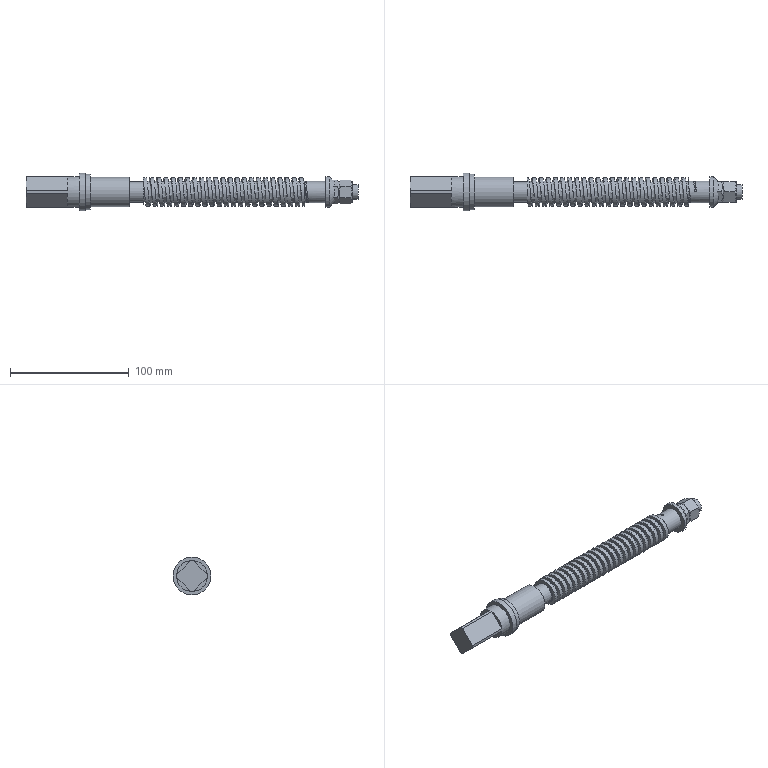Part | NX | features DATUM_CSYS 9, CYLINDER 8, SKETCH 6, EXTRUDE 4, SYMBOLIC_THREAD 3, EXTRACT_DATUM_AXIS 2, EXTRACT_STRING 2, HOLE PACKAGE 2, RECT_GROOVE 2, SIMPLE HOLE 2, SWP104 2, THREADS 2, CHAMFER 1, CONE 1, DATUM_ON_PATH 1, DELETE FACE 1, HELIX 1, INTERSECT 1, Instance Feature 1, Mirror Feature 1, SKIN 1, SUBTRACT 1 | 4 solids | 83 faces | box 280 x 32 x 32 mm | volume 105505 mm3 | plane 39 | cone 18 | cylinder 17 | spline 9 | commonest cylinder face diameters 18 x3 10.3 x2 12 x2 26 x2 9 x1 12.423 x1